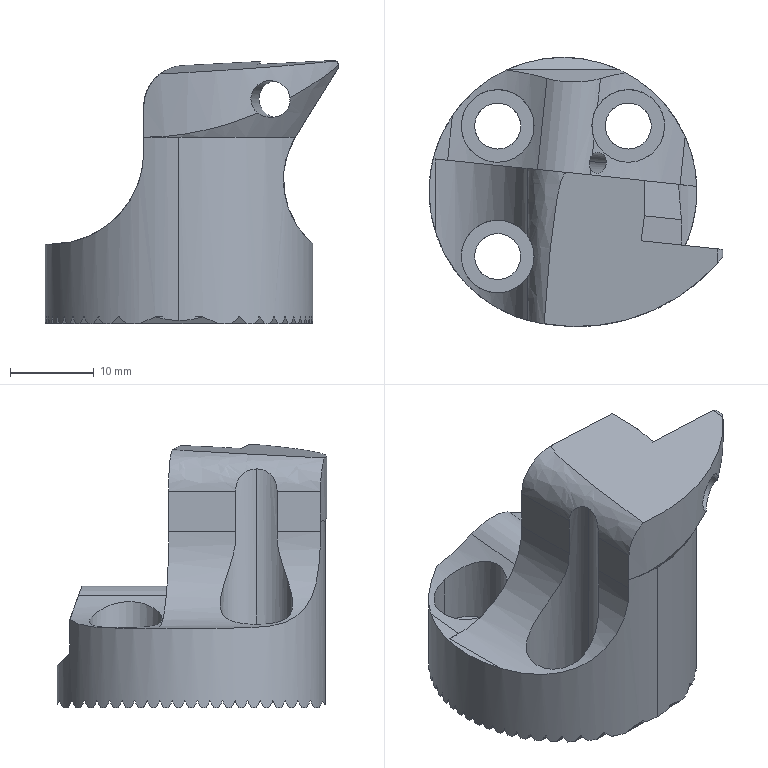NC program | Mastercam | posted with a generic post
Whole program:
%
:0001()
(MATERIAL - ALUMINUM MM - 2024)
(T8|25 60DTH |H8|D8|WEAR COMP|TOOL DIA. - 25.)
(T5|8 FEMR |H5|D5|WEAR COMP|TOOL DIA. - 8.|XY STOCK TO LEAVE - .1|Z STOCK TO LEAVE - 0.)
(T6|8 FEMF |H6|D6|WEAR COMP|TOOL DIA. - 8.|XY STOCK TO LEAVE - .05|Z STOCK TO LEAVE - 0.)
(T3|10 SPD |H3)
(T9|8.7 CBDR |H9)
(T12|8.7 CBFL |H12)
N100 G21
N102 G0 G17 G40 G80 G90 G94 G98
N104 G0 G28 G91 Z0.
N106 G0 G28 X0. Y0.
(25 60DTH |TOOL - 8|DIA. OFF. - 8|LEN. - 8|TOOL DIA. - 25.)
N108 T8 M6
N110 G0 G54 G90 X-15.8 Y-4.917 C180. B-90. S4000 M3
N112 G43 H8 Z100.
N114 Z15.75
N116 G1 Z10.75 F2000.
N118 G41 D8 X-11.8 F1000.
N120 G3 X-11.7 Y-4.817 J.1
N122 G1 Y-2.817
N124 Y2.817
N126 Y4.817
N128 G3 X-11.8 Y4.917 I-.1
N130 G1 G40 X-15.8
N132 G0 Z25.75
N134 Y-9.376
N136 Z14.25
N138 G1 Z9.25 F2000.
N140 G41 D8 X-11.8 F1000.
N142 G3 X-11.7 Y-9.276 J.1
N144 G1 Y-7.276
N146 Y7.276
N148 Y9.276
N150 G3 X-11.8 Y9.376 I-.1
N152 G1 G40 X-15.8
N154 G0 Z24.25
N156 Y-11.766
N158 Z12.75
N160 G1 Z7.75 F2000.
N162 G41 D8 X-11.8 F1000.
N164 G3 X-11.7 Y-11.666 J.1
N166 G1 Y-9.666
N168 Y9.666
N170 Y11.666
N172 G3 X-11.8 Y11.766 I-.1
N174 G1 G40 X-15.8
N176 G0 Z22.75
N178 Y-13.477
N180 Z11.25
N182 G1 Z6.25 F2000.
N184 G41 D8 X-11.8 F1000.
N186 G3 X-11.7 Y-13.377 J.1
N188 G1 Y-11.377
N190 Y11.377
N192 Y13.377
N194 G3 X-11.8 Y13.477 I-.1
N196 G1 G40 X-15.8
N198 G0 Z21.25
N200 Y-14.786
N202 Z9.75
N204 G1 Z4.75 F2000.
N206 G41 D8 X-11.8 F1000.
N208 G3 X-11.7 Y-14.686 J.1
N210 G1 Y-12.686
N212 Y12.686
N214 Y14.686
N216 G3 X-11.8 Y14.786 I-.1
N218 G1 G40 X-15.8
N220 G0 Z19.75
N222 Y-15.809
N224 Z8.25
N226 G1 Z3.25 F2000.
N228 G41 D8 X-11.8 F1000.
N230 G3 X-11.7 Y-15.709 J.1
N232 G1 Y-13.709
N234 Y13.709
N236 Y15.709
N238 G3 X-11.8 Y15.809 I-.1
N240 G1 G40 X-15.8
N242 G0 Z18.25
N244 Y-16.606
N246 Z6.75
N248 G1 Z1.75 F2000.
N250 G41 D8 X-11.8 F1000.
N252 G3 X-11.7 Y-16.506 J.1
N254 G1 Y-14.506
N256 Y14.506
N258 Y16.506
N260 G3 X-11.8 Y16.606 I-.1
N262 G1 G40 X-15.8
N264 G0 Z16.75
N266 Y-17.214
N268 Z5.25
N270 G1 Z.25 F2000.
N272 G41 D8 X-11.8 F1000.
N274 G3 X-11.7 Y-17.114 J.1
N276 G1 Y-15.114
N278 Y15.114
N280 Y17.114
N282 G3 X-11.8 Y17.214 I-.1
N284 G1 G40 X-15.8
N286 G0 Z15.25
N288 Y-17.654
N290 Z3.75
N292 G1 Z-1.25 F2000.
N294 G41 D8 X-11.8 F1000.
N296 G3 X-11.7 Y-17.554 J.1
N298 G1 Y-15.554
N300 Y15.554
N302 Y17.554
N304 G3 X-11.8 Y17.654 I-.1
N306 G1 G40 X-15.8
N308 G0 Z13.75
N310 Y-17.941
N312 Z2.25
N314 G1 Z-2.75 F2000.
N316 G41 D8 X-11.8 F1000.
N318 G3 X-11.7 Y-17.841 J.1
N320 G1 Y-15.841
N322 Y15.841
N324 Y17.841
N326 G3 X-11.8 Y17.941 I-.1
N328 G1 G40 X-15.8
N330 G0 Z12.25
N332 Y-18.082
N334 Z.75
N336 G1 Z-4.25 F2000.
N338 G41 D8 X-11.8 F1000.
N340 G3 X-11.7 Y-17.982 J.1
N342 G1 Y-15.982
N344 Y15.982
N346 Y17.982
N348 G3 X-11.8 Y18.082 I-.1
N350 G1 G40 X-15.8
N352 G0 Z10.75
N354 Y-18.082
N356 Z-.75
N358 G1 Z-5.75 F2000.
N360 G41 D8 X-11.8 F1000.
N362 G3 X-11.7 Y-17.982 J.1
N364 G1 Y-15.982
N366 Y15.982
N368 Y17.982
N370 G3 X-11.8 Y18.082 I-.1
N372 G1 G40 X-15.8
N374 G0 Z9.25
N376 Y-17.941
N378 Z-2.25
N380 G1 Z-7.25 F2000.
N382 G41 D8 X-11.8 F1000.
N384 G3 X-11.7 Y-17.841 J.1
N386 G1 Y-15.841
N388 Y15.841
N390 Y17.841
N392 G3 X-11.8 Y17.941 I-.1
N394 G1 G40 X-15.8
N396 G0 Z7.75
N398 Y-17.654
N400 Z-3.75
N402 G1 Z-8.75 F2000.
N404 G41 D8 X-11.8 F1000.
N406 G3 X-11.7 Y-17.554 J.1
N408 G1 Y-15.554
N410 Y15.554
N412 Y17.554
N414 G3 X-11.8 Y17.654 I-.1
N416 G1 G40 X-15.8
N418 G0 Z6.25
N420 Y-17.214
N422 Z-5.25
N424 G1 Z-10.25 F2000.
N426 G41 D8 X-11.8 F1000.
N428 G3 X-11.7 Y-17.114 J.1
N430 G1 Y-15.114
N432 Y-6.77
N434 Y15.114
N436 Y17.114
N438 G3 X-11.8 Y17.214 I-.1
N440 G1 G40 X-15.8
N442 G0 Z4.75
N444 Y-16.606
N446 Z-6.75
N448 G1 Z-11.75 F2000.
N450 G41 D8 X-11.8 F1000.
N452 G3 X-11.7 Y-16.506 J.1
N454 G1 Y-14.506
N456 Y14.506
N458 Y16.506
N460 G3 X-11.8 Y16.606 I-.1
N462 G1 G40 X-15.8
N464 G0 Z3.25
N466 Y-15.809
N468 Z-8.25
N470 G1 Z-13.25 F2000.
N472 G41 D8 X-11.8 F1000.
N474 G3 X-11.7 Y-15.709 J.1
N476 G1 Y-13.709
N478 Y13.709
N480 Y15.709
N482 G3 X-11.8 Y15.809 I-.1
N484 G1 G40 X-15.8
N486 G0 Z1.75
N488 Y-14.786
N490 Z-9.75
N492 G1 Z-14.75 F2000.
N494 G41 D8 X-11.8 F1000.
N496 G3 X-11.7 Y-14.686 J.1
N498 G1 Y-12.686
N500 Y12.686
N502 Y14.686
N504 G3 X-11.8 Y14.786 I-.1
N506 G1 G40 X-15.8
N508 G0 Z.25
N510 Y-13.477
N512 Z-11.25
N514 G1 Z-16.25 F2000.
N516 G41 D8 X-11.8 F1000.
N518 G3 X-11.7 Y-13.377 J.1
N520 G1 Y-11.377
N522 Y11.377
N524 Y13.377
N526 G3 X-11.8 Y13.477 I-.1
N528 G1 G40 X-15.8
N530 G0 Z-1.25
N532 Y-11.766
N534 Z-12.75
N536 G1 Z-17.75 F2000.
N538 G41 D8 X-11.8 F1000.
N540 G3 X-11.7 Y-11.666 J.1
N542 G1 Y-9.666
N544 Y9.666
N546 Y11.666
N548 G3 X-11.8 Y11.766 I-.1
N550 G1 G40 X-15.8
N552 G0 Z-2.75
N554 Y-9.376
N556 Z-14.25
N558 G1 Z-19.25 F2000.
N560 G41 D8 X-11.8 F1000.
N562 G3 X-11.7 Y-9.276 J.1
N564 G1 Y-7.276
N566 Y7.276
N568 Y9.276
N570 G3 X-11.8 Y9.376 I-.1
N572 G1 G40 X-15.8
N574 G0 Z-4.25
N576 Y-4.917
N578 Z-15.75
N580 G1 Z-20.75 F2000.
N582 G41 D8 X-11.8 F1000.
N584 G3 X-11.7 Y-4.817 J.1
N586 G1 Y-2.817
N588 Y2.817
N590 Y4.817
N592 G3 X-11.8 Y4.917 I-.1
N594 G1 G40 X-15.8
N596 G0 Z100.
N598 M5
N600 G0 G28 G91 Z0.
N602 G28 C0. B0.
N604 M01
N606 G0 G17 G40 G80 G90 G94 G98
N608 G0 G28 G91 Z0.
(8 FEMR |TOOL - 5|DIA. OFF. - 5|LEN. - 5|TOOL DIA. - 8.)
N610 T5 M6
N612 G0 G54 G90 X0. Y0. C0. B180. S3500 M3
N614 G43 H5 Z50.
N616 Z2.
N618 G1 Z-4. F2000.
N620 G41 D5 X-1.316 F400.
N622 G3 X-1.358 Y-.239 I.658 J-.239
N624 X-1.316 Y-.479 I.7
N626 X0. Y-1.4 I1.316 J.479
N628 X1.4 Y0. J1.4
N630 X0. Y1.4 I-1.4
N632 X-1.4 Y0. J-1.4
N634 X-1.316 Y-.479 I1.4
N636 X-1.266 Y-.598 I1.316 J.479
N638 X-.925 Y-.935 I.633 J.299
N640 G1 G40 X0. Y0.
N642 G41 D5 X-1.55
N644 G3 X-1.6 Y-.282 I.775 J-.282
N646 X-1.55 Y-.564 I.825
N648 X0. Y-1.649 I1.55 J.564
N650 X1.649 Y0. J1.649
N652 X0. Y1.649 I-1.649
N654 X-1.649 Y0. J-1.649
N656 X-1.55 Y-.564 I1.649
N658 X-1.495 Y-.699 I1.55 J.564
N660 X-1.095 Y-1.098 I.748 J.349
N662 G1 G40 X0. Y0.
N664 G41 D5 X-1.785
N666 G3 X-1.842 Y-.325 I.892 J-.325
N668 X-1.785 Y-.65 I.949
N670 X0. Y-1.9 I1.785 J.65
N672 X1.9 Y0. J1.9
N674 X0. Y1.9 I-1.9
N676 X-1.9 Y0. J-1.9
N678 X-1.785 Y-.65 I1.9
N680 X-1.724 Y-.799 I1.785 J.65
N682 X-1.266 Y-1.259 I.862 J.4
N684 G1 G40 X0. Y0.
N686 G0 Z50.
N688 M5
N690 G0 G28 G91 Z0.
N692 G28 B0.
N694 M01
N696 G0 G17 G40 G80 G90 G94 G98
N698 G0 G28 G91 Z0.
(8 FEMF |TOOL - 6|DIA. OFF. - 6|LEN. - 6|TOOL DIA. - 8.)
N700 T6 M6
N702 G0 G54 G90 X0. Y0. C0. B180. S3500 M3
N704 G43 H6 Z50.
N706 Z2.
N708 G1 Z-4. F2000.
N710 G41 D6 X-1.832 F400.
N712 G3 X-1.891 Y-.333 I.916 J-.333
N714 X-1.832 Y-.667 I.975
N716 X0. Y-1.95 I1.832 J.667
N718 X1.95 Y0. J1.95
N720 X0. Y1.95 I-1.95
N722 X-1.95 Y0. J-1.95
N724 X-1.832 Y-.667 I1.95
N726 X-1.77 Y-.818 I1.832 J.667
N728 X-1.3 Y-1.292 I.885 J.409
N730 G1 G40 X0. Y0.
N732 G41 D6 X-1.832
N734 G3 X-1.891 Y-.333 I.916 J-.333
N736 X-1.832 Y-.667 I.975
N738 X0. Y-1.95 I1.832 J.667
N740 X1.95 Y0. J1.95
N742 X0. Y1.95 I-1.95
N744 X-1.95 Y0. J-1.95
N746 X-1.832 Y-.667 I1.95
N748 X-1.77 Y-.818 I1.832 J.667
N750 X-1.3 Y-1.292 I.885 J.409
N752 G1 G40 X0. Y0.
N754 G41 D6 X-1.832
N756 G3 X-1.891 Y-.333 I.916 J-.333
N758 X-1.832 Y-.667 I.975
N760 X0. Y-1.95 I1.832 J.667
N762 X1.95 Y0. J1.95
N764 X0. Y1.95 I-1.95
N766 X-1.95 Y0. J-1.95
N768 X-1.832 Y-.667 I1.95
N770 X-1.77 Y-.818 I1.832 J.667
N772 X-1.3 Y-1.292 I.885 J.409
N774 G1 G40 X0. Y0.
N776 G0 Z50.
N778 M5
N780 G0 G28 G91 Z0.
N782 G28 B0.
N784 M01
N786 G0 G17 G40 G80 G90 G94 G98
N788 G0 G28 G91 Z0.
(10 SPD |TOOL - 3|DIA. OFF. - 3|LEN. - 3|TOOL DIA. - 10.)
N790 T3 M6
N792 G0 G54 G90 X-7.8 Y7.8 C0. B0. S2000 M3
N794 G43 H3 Z85.
N796 G81 G98 Z33. R36. F100.
N798 X7.8
N800 X-7.8 Y-7.8
N802 G80
N804 M5
N806 G0 G28 G91 Z0.
N808 G28
N810 M01
N812 G0 G17 G40 G80 G90 G94 G98
N814 G0 G28 G91 Z0.
(8.7 CBDR |TOOL - 9|DIA. OFF. - 9|LEN. - 9|TOOL DIA. - 8.7)
N816 T9 M6
N818 G0 G54 G90 X-7.8 Y7.8 C0. B0. S2000 M3
N820 G43 H9 Z85.
N822 G83 G98 Z2.5 R36. Q4. F100.
N824 X7.8
N826 X-7.8 Y-7.8
N828 G80
N830 M5
N832 G0 G28 G91 Z0.
N834 G28
N836 M01
N838 G0 G17 G40 G80 G90 G94 G98
N840 G0 G28 G91 Z0.
(8.7 CBFL |TOOL - 12|DIA. OFF. - 12|LEN. - 12|TOOL DIA. - 8.7)
N842 T12 M6
N844 G0 G54 G90 X-7.8 Y7.8 C0. B0. S2000 M3
N846 G43 H12 Z85.
N848 G82 G98 Z4. R7. P1. F100.
N850 X7.8 P1.
N852 X-7.8 Y-7.8 P1.
N854 G80
N856 M5
N858 G0 G28 G91 Z0.
N860 G0 G28 X0. Y0.
N862 G28
N864 M30
%